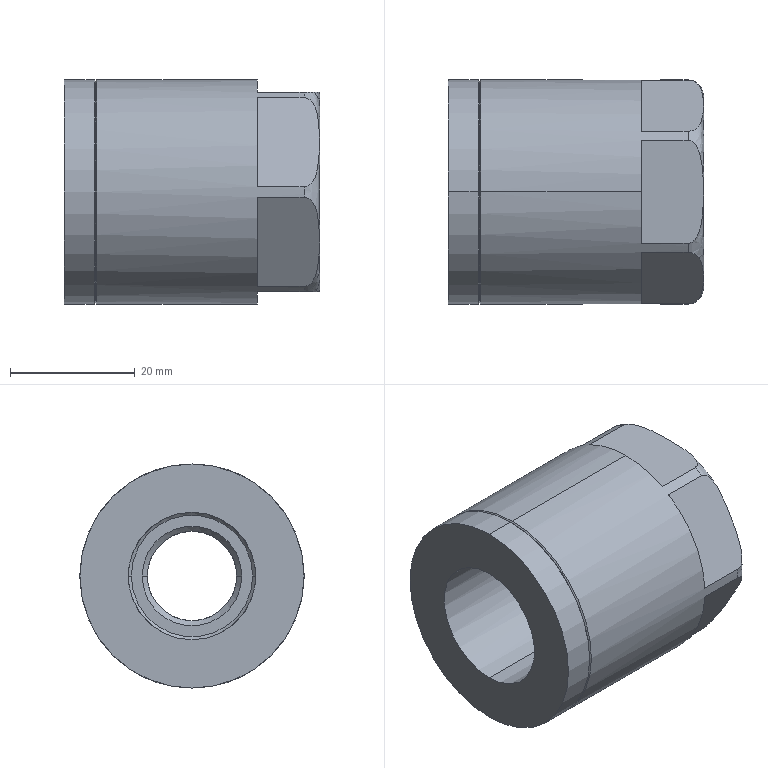Part | SolidWorks | features BaseBody 1 | 1 solid | 35 faces | box 41 x 36 x 36 mm | volume 28650 mm3 | plane 15 | cone 10 | cylinder 8 | spline 2 | commonest cylinder face diameters 36 x4 14.376 x2 20.5 x2
STEP:
#1=CARTESIAN_POINT('',(41.,0.,-15.5));
#2=VERTEX_POINT('',#1);
#3=CARTESIAN_POINT('',(41.,0.,15.5));
#4=VERTEX_POINT('',#3);
#5=CARTESIAN_POINT('',(41.,0.,-15.5));
#6=CARTESIAN_POINT('',(41.,-31.,-15.5));
#7=CARTESIAN_POINT('',(41.,-31.,15.5));
#8=CARTESIAN_POINT('',(41.,0.,15.5));
#9=(BOUNDED_CURVE()B_SPLINE_CURVE(3,(#5,#6,#7,#8),.UNSPECIFIED.,.F.,.F.)B_SPLINE_CURVE_WITH_KNOTS((4,4),(0.,0.5),.UNSPECIFIED.)CURVE()GEOMETRIC_REPRESENTATION_ITEM()RATIONAL_B_SPLINE_CURVE((1.,0.3333,0.3333,1.))REPRESENTATION_ITEM(''));
#10=EDGE_CURVE('',#2,#4,#9,.T.);
#11=ORIENTED_EDGE('',*,*,#10,.T.);
#12=CARTESIAN_POINT('',(40.949,0.,16.));
#13=VERTEX_POINT('',#12);
#14=CARTESIAN_POINT('',(38.5,0.,15.5));
#15=DIRECTION('',(0.,-1.,0.));
#16=DIRECTION('',(0.,0.,1.));
#17=AXIS2_PLACEMENT_3D('',#14,#15,#16);
#18=CIRCLE('',#17,2.5);
#19=EDGE_CURVE('',#4,#13,#18,.T.);
#20=ORIENTED_EDGE('',*,*,#19,.T.);
#21=CARTESIAN_POINT('',(38.5,-8.246,16.));
#22=VERTEX_POINT('',#21);
#23=CARTESIAN_POINT('',(38.5,-8.246,16.));
#24=CARTESIAN_POINT('',(38.598,-8.246,16.));
#25=CARTESIAN_POINT('',(38.694,-8.234,16.));
#26=CARTESIAN_POINT('',(38.882,-8.186,16.));
#27=CARTESIAN_POINT('',(38.974,-8.151,16.));
#28=CARTESIAN_POINT('',(39.233,-8.019,16.));
#29=CARTESIAN_POINT('',(39.388,-7.896,16.));
#30=CARTESIAN_POINT('',(39.657,-7.62,16.));
#31=CARTESIAN_POINT('',(39.774,-7.463,16.));
#32=CARTESIAN_POINT('',(39.98,-7.137,16.));
#33=CARTESIAN_POINT('',(40.068,-6.966,16.));
#34=CARTESIAN_POINT('',(40.303,-6.439,16.));
#35=CARTESIAN_POINT('',(40.42,-6.068,16.));
#36=CARTESIAN_POINT('',(40.604,-5.326,16.));
#37=CARTESIAN_POINT('',(40.671,-4.951,16.));
#38=CARTESIAN_POINT('',(40.831,-3.82,16.));
#39=CARTESIAN_POINT('',(40.881,-3.056,16.));
#40=CARTESIAN_POINT('',(40.94,-1.527,16.));
#41=CARTESIAN_POINT('',(40.949,-0.763,16.));
#42=CARTESIAN_POINT('',(40.949,0.,16.));
#43=B_SPLINE_CURVE_WITH_KNOTS('',3,(#23,#24,#25,#26,#27,#28,#29,#30,#31,#32,#33,#34,#35,#36,#37,#38,#39,#40,#41,#42),.UNSPECIFIED.,.F.,.F.,(4,2,2,2,2,2,2,2,2,4),(0.,0.0002896,0.0005792,0.001158,0.001738,0.002317,0.003475,0.004634,0.006951,0.009268),.UNSPECIFIED.);
#44=EDGE_CURVE('',#22,#13,#43,.T.);
#45=ORIENTED_EDGE('',*,*,#44,.F.);
#46=CARTESIAN_POINT('',(38.5,-9.733,15.141));
#47=VERTEX_POINT('',#46);
#48=CARTESIAN_POINT('',(38.5,0.,0.));
#49=DIRECTION('',(1.,0.,0.));
#50=DIRECTION('',(0.,0.,-1.));
#51=AXIS2_PLACEMENT_3D('',#48,#49,#50);
#52=CIRCLE('',#51,18.);
#53=EDGE_CURVE('',#22,#47,#52,.T.);
#54=ORIENTED_EDGE('',*,*,#53,.T.);
#55=CARTESIAN_POINT('',(38.5,-17.98,0.8586));
#56=VERTEX_POINT('',#55);
#57=CARTESIAN_POINT('',(38.5,-17.98,0.8586));
#58=CARTESIAN_POINT('',(38.598,-17.98,0.8586));
#59=CARTESIAN_POINT('',(38.694,-17.973,0.8694));
#60=CARTESIAN_POINT('',(38.881,-17.95,0.9105));
#61=CARTESIAN_POINT('',(38.973,-17.932,0.9412));
#62=CARTESIAN_POINT('',(39.232,-17.866,1.055));
#63=CARTESIAN_POINT('',(39.386,-17.805,1.161));
#64=CARTESIAN_POINT('',(39.655,-17.667,1.4));
#65=CARTESIAN_POINT('',(39.773,-17.589,1.535));
#66=CARTESIAN_POINT('',(39.978,-17.426,1.817));
#67=CARTESIAN_POINT('',(40.066,-17.341,1.964));
#68=CARTESIAN_POINT('',(40.302,-17.078,2.42));
#69=CARTESIAN_POINT('',(40.419,-16.893,2.74));
#70=CARTESIAN_POINT('',(40.602,-16.523,3.382));
#71=CARTESIAN_POINT('',(40.67,-16.336,3.706));
#72=CARTESIAN_POINT('',(40.83,-15.771,4.684));
#73=CARTESIAN_POINT('',(40.88,-15.389,5.345));
#74=CARTESIAN_POINT('',(40.94,-14.626,6.667));
#75=CARTESIAN_POINT('',(40.949,-14.245,7.327));
#76=CARTESIAN_POINT('',(40.95,-13.483,8.646));
#77=CARTESIAN_POINT('',(40.941,-13.103,9.305));
#78=CARTESIAN_POINT('',(40.882,-12.343,10.622));
#79=CARTESIAN_POINT('',(40.834,-11.963,11.28));
#80=CARTESIAN_POINT('',(40.676,-11.395,12.263));
#81=CARTESIAN_POINT('',(40.609,-11.207,12.59));
#82=CARTESIAN_POINT('',(40.425,-10.83,13.241));
#83=CARTESIAN_POINT('',(40.309,-10.644,13.564));
#84=CARTESIAN_POINT('',(40.072,-10.377,14.026));
#85=CARTESIAN_POINT('',(39.983,-10.291,14.175));
#86=CARTESIAN_POINT('',(39.779,-10.128,14.457));
#87=CARTESIAN_POINT('',(39.664,-10.051,14.591));
#88=CARTESIAN_POINT('',(39.392,-9.91,14.835));
#89=CARTESIAN_POINT('',(39.237,-9.848,14.942));
#90=CARTESIAN_POINT('',(38.976,-9.782,15.058));
#91=CARTESIAN_POINT('',(38.886,-9.764,15.088));
#92=CARTESIAN_POINT('',(38.698,-9.74,15.13));
#93=CARTESIAN_POINT('',(38.599,-9.733,15.141));
#94=CARTESIAN_POINT('',(38.5,-9.733,15.141));
#95=B_SPLINE_CURVE_WITH_KNOTS('',3,(#57,#58,#59,#60,#61,#62,#63,#64,#65,#66,#67,#68,#69,#70,#71,#72,#73,#74,#75,#76,#77,#78,#79,#80,#81,#82,#83,#84,#85,#86,#87,#88,#89,#90,#91,#92,#93,#94),.UNSPECIFIED.,.F.,.F.,(4,2,2,2,2,2,2,2,2,2,2,2,2,2,2,2,2,2,4),(0.,0.0002891,0.0005782,0.001156,0.001735,0.002313,0.003469,0.004626,0.006939,0.009252,0.01156,0.01388,0.01503,0.01619,0.01677,0.01735,0.01792,0.01821,0.0185),.UNSPECIFIED.);
#96=EDGE_CURVE('',#56,#47,#95,.T.);
#97=ORIENTED_EDGE('',*,*,#96,.F.);
#98=CARTESIAN_POINT('',(38.5,-17.98,-0.8586));
#99=VERTEX_POINT('',#98);
#100=CARTESIAN_POINT('',(38.5,0.,0.));
#101=DIRECTION('',(1.,0.,0.));
#102=DIRECTION('',(0.,0.,-1.));
#103=AXIS2_PLACEMENT_3D('',#100,#101,#102);
#104=CIRCLE('',#103,18.);
#105=EDGE_CURVE('',#56,#99,#104,.T.);
#106=ORIENTED_EDGE('',*,*,#105,.T.);
#107=CARTESIAN_POINT('',(38.5,-9.733,-15.141));
#108=VERTEX_POINT('',#107);
#109=CARTESIAN_POINT('',(38.5,-9.733,-15.141));
#110=CARTESIAN_POINT('',(38.598,-9.733,-15.141));
#111=CARTESIAN_POINT('',(38.694,-9.74,-15.131));
#112=CARTESIAN_POINT('',(38.881,-9.763,-15.09));
#113=CARTESIAN_POINT('',(38.973,-9.781,-15.059));
#114=CARTESIAN_POINT('',(39.232,-9.847,-14.945));
#115=CARTESIAN_POINT('',(39.386,-9.908,-14.839));
#116=CARTESIAN_POINT('',(39.655,-10.046,-14.6));
#117=CARTESIAN_POINT('',(39.773,-10.124,-14.465));
#118=CARTESIAN_POINT('',(39.978,-10.287,-14.183));
#119=CARTESIAN_POINT('',(40.066,-10.372,-14.036));
#120=CARTESIAN_POINT('',(40.302,-10.635,-13.58));
#121=CARTESIAN_POINT('',(40.419,-10.82,-13.26));
#122=CARTESIAN_POINT('',(40.602,-11.19,-12.618));
#123=CARTESIAN_POINT('',(40.67,-11.377,-12.294));
#124=CARTESIAN_POINT('',(40.83,-11.942,-11.316));
#125=CARTESIAN_POINT('',(40.88,-12.323,-10.655));
#126=CARTESIAN_POINT('',(40.94,-13.087,-9.333));
#127=CARTESIAN_POINT('',(40.949,-13.468,-8.673));
#128=CARTESIAN_POINT('',(40.95,-14.229,-7.354));
#129=CARTESIAN_POINT('',(40.941,-14.61,-6.695));
#130=CARTESIAN_POINT('',(40.882,-15.37,-5.378));
#131=CARTESIAN_POINT('',(40.834,-15.75,-4.72));
#132=CARTESIAN_POINT('',(40.676,-16.317,-3.737));
#133=CARTESIAN_POINT('',(40.609,-16.506,-3.41));
#134=CARTESIAN_POINT('',(40.425,-16.883,-2.759));
#135=CARTESIAN_POINT('',(40.309,-17.069,-2.436));
#136=CARTESIAN_POINT('',(40.072,-17.336,-1.974));
#137=CARTESIAN_POINT('',(39.983,-17.421,-1.825));
#138=CARTESIAN_POINT('',(39.779,-17.584,-1.543));
#139=CARTESIAN_POINT('',(39.664,-17.662,-1.409));
#140=CARTESIAN_POINT('',(39.392,-17.803,-1.165));
#141=CARTESIAN_POINT('',(39.237,-17.864,-1.058));
#142=CARTESIAN_POINT('',(38.976,-17.931,-0.9423));
#143=CARTESIAN_POINT('',(38.886,-17.949,-0.9119));
#144=CARTESIAN_POINT('',(38.698,-17.973,-0.8699));
#145=CARTESIAN_POINT('',(38.599,-17.98,-0.8586));
#146=CARTESIAN_POINT('',(38.5,-17.98,-0.8586));
#147=B_SPLINE_CURVE_WITH_KNOTS('',3,(#109,#110,#111,#112,#113,#114,#115,#116,#117,#118,#119,#120,#121,#122,#123,#124,#125,#126,#127,#128,#129,#130,#131,#132,#133,#134,#135,#136,#137,#138,#139,#140,#141,#142,#143,#144,#145,#146),.UNSPECIFIED.,.F.,.F.,(4,2,2,2,2,2,2,2,2,2,2,2,2,2,2,2,2,2,4),(0.,0.0002891,0.0005782,0.001156,0.001735,0.002313,0.003469,0.004626,0.006939,0.009252,0.01156,0.01388,0.01503,0.01619,0.01677,0.01735,0.01792,0.01821,0.0185),.UNSPECIFIED.);
#148=EDGE_CURVE('',#108,#99,#147,.T.);
#149=ORIENTED_EDGE('',*,*,#148,.F.);
#150=CARTESIAN_POINT('',(38.5,-8.246,-16.));
#151=VERTEX_POINT('',#150);
#152=CARTESIAN_POINT('',(38.5,0.,0.));
#153=DIRECTION('',(1.,0.,0.));
#154=DIRECTION('',(0.,0.,-1.));
#155=AXIS2_PLACEMENT_3D('',#152,#153,#154);
#156=CIRCLE('',#155,18.);
#157=EDGE_CURVE('',#108,#151,#156,.T.);
#158=ORIENTED_EDGE('',*,*,#157,.T.);
#159=CARTESIAN_POINT('',(40.949,0.,-16.));
#160=VERTEX_POINT('',#159);
#161=CARTESIAN_POINT('',(40.949,0.,-16.));
#162=CARTESIAN_POINT('',(40.949,-0.7604,-16.));
#163=CARTESIAN_POINT('',(40.94,-1.52,-16.));
#164=CARTESIAN_POINT('',(40.882,-3.038,-16.));
#165=CARTESIAN_POINT('',(40.833,-3.796,-16.));
#166=CARTESIAN_POINT('',(40.675,-4.929,-16.));
#167=CARTESIAN_POINT('',(40.608,-5.306,-16.));
#168=CARTESIAN_POINT('',(40.423,-6.058,-16.));
#169=CARTESIAN_POINT('',(40.307,-6.429,-16.));
#170=CARTESIAN_POINT('',(40.07,-6.962,-16.));
#171=CARTESIAN_POINT('',(39.982,-7.133,-16.));
#172=CARTESIAN_POINT('',(39.778,-7.458,-16.));
#173=CARTESIAN_POINT('',(39.663,-7.612,-16.));
#174=CARTESIAN_POINT('',(39.391,-7.893,-16.));
#175=CARTESIAN_POINT('',(39.236,-8.017,-16.));
#176=CARTESIAN_POINT('',(38.975,-8.15,-16.));
#177=CARTESIAN_POINT('',(38.885,-8.185,-16.));
#178=CARTESIAN_POINT('',(38.697,-8.233,-16.));
#179=CARTESIAN_POINT('',(38.599,-8.246,-16.));
#180=CARTESIAN_POINT('',(38.5,-8.246,-16.));
#181=B_SPLINE_CURVE_WITH_KNOTS('',3,(#161,#162,#163,#164,#165,#166,#167,#168,#169,#170,#171,#172,#173,#174,#175,#176,#177,#178,#179,#180),.UNSPECIFIED.,.F.,.F.,(4,2,2,2,2,2,2,2,2,4),(0.009268,0.01158,0.01389,0.01504,0.01619,0.01677,0.01735,0.01793,0.01821,0.0185),.UNSPECIFIED.);
#182=EDGE_CURVE('',#160,#151,#181,.T.);
#183=ORIENTED_EDGE('',*,*,#182,.F.);
#184=CARTESIAN_POINT('',(38.5,0.,-15.5));
#185=DIRECTION('',(0.,1.,0.));
#186=DIRECTION('',(0.,0.,-1.));
#187=AXIS2_PLACEMENT_3D('',#184,#185,#186);
#188=CIRCLE('',#187,2.5);
#189=EDGE_CURVE('',#2,#160,#188,.T.);
#190=ORIENTED_EDGE('',*,*,#189,.F.);
#191=EDGE_LOOP('',(#11,#20,#45,#54,#97,#106,#149,#158,#183,#190));
#192=FACE_OUTER_BOUND('',#191,.T.);
#193=CARTESIAN_POINT('',(40.994,0.,15.334));
#194=CARTESIAN_POINT('',(40.994,-30.667,15.334));
#195=CARTESIAN_POINT('',(40.994,-30.667,-15.334));
#196=CARTESIAN_POINT('',(40.994,0.,-15.334));
#197=CARTESIAN_POINT('',(41.097,0.,16.873));
#198=CARTESIAN_POINT('',(41.097,-33.746,16.873));
#199=CARTESIAN_POINT('',(41.097,-33.746,-16.873));
#200=CARTESIAN_POINT('',(41.097,0.,-16.873));
#201=CARTESIAN_POINT('',(40.043,0.,18.));
#202=CARTESIAN_POINT('',(40.043,-36.,18.));
#203=CARTESIAN_POINT('',(40.043,-36.,-18.));
#204=CARTESIAN_POINT('',(40.043,0.,-18.));
#205=CARTESIAN_POINT('',(38.5,0.,18.));
#206=CARTESIAN_POINT('',(38.5,-36.,18.));
#207=CARTESIAN_POINT('',(38.5,-36.,-18.));
#208=CARTESIAN_POINT('',(38.5,0.,-18.));
#209=(BOUNDED_SURFACE()B_SPLINE_SURFACE(3,3,((#193,#194,#195,#196),(#197,#198,#199,#200),(#201,#202,#203,#204),(#205,#206,#207,#208)),.UNSPECIFIED.,.F.,.F.,.T.)B_SPLINE_SURFACE_WITH_KNOTS((4,4),(4,4),(0.,1.),(0.,1.),.UNSPECIFIED.)GEOMETRIC_REPRESENTATION_ITEM()RATIONAL_B_SPLINE_SURFACE(((1.,0.3333,0.3333,1.),(0.7888,0.2629,0.2629,0.7888),(0.7888,0.2629,0.2629,0.7888),(1.,0.3333,0.3333,1.)))REPRESENTATION_ITEM('')SURFACE());
#210=ADVANCED_FACE('',(#192),#209,.T.);
#211=CARTESIAN_POINT('',(31.,8.246,-16.));
#212=VERTEX_POINT('',#211);
#213=CARTESIAN_POINT('',(31.,0.,-18.));
#214=VERTEX_POINT('',#213);
#215=CARTESIAN_POINT('',(31.,0.,0.));
#216=DIRECTION('',(-1.,0.,0.));
#217=DIRECTION('',(0.,0.,1.));
#218=AXIS2_PLACEMENT_3D('',#215,#216,#217);
#219=CIRCLE('',#218,18.);
#220=EDGE_CURVE('',#212,#214,#219,.T.);
#221=ORIENTED_EDGE('',*,*,#220,.T.);
#222=CARTESIAN_POINT('',(5.2,0.,-18.));
#223=VERTEX_POINT('',#222);
#224=CARTESIAN_POINT('',(41.,0.,-18.));
#225=DIRECTION('',(-1.,0.,0.));
#226=VECTOR('',#225,1000.);
#227=LINE('',#224,#226);
#228=EDGE_CURVE('',#214,#223,#227,.T.);
#229=ORIENTED_EDGE('',*,*,#228,.T.);
#230=CARTESIAN_POINT('',(5.2,0.,18.));
#231=VERTEX_POINT('',#230);
#232=CARTESIAN_POINT('',(5.2,0.,0.));
#233=DIRECTION('',(1.,0.,0.));
#234=DIRECTION('',(0.,0.,1.));
#235=AXIS2_PLACEMENT_3D('',#232,#233,#234);
#236=CIRCLE('',#235,18.);
#237=EDGE_CURVE('',#223,#231,#236,.T.);
#238=ORIENTED_EDGE('',*,*,#237,.T.);
#239=CARTESIAN_POINT('',(31.,0.,18.));
#240=VERTEX_POINT('',#239);
#241=CARTESIAN_POINT('',(41.,0.,18.));
#242=DIRECTION('',(-1.,0.,0.));
#243=VECTOR('',#242,1000.);
#244=LINE('',#241,#243);
#245=EDGE_CURVE('',#240,#231,#244,.T.);
#246=ORIENTED_EDGE('',*,*,#245,.F.);
#247=CARTESIAN_POINT('',(31.,8.246,16.));
#248=VERTEX_POINT('',#247);
#249=CARTESIAN_POINT('',(31.,0.,0.));
#250=DIRECTION('',(-1.,0.,0.));
#251=DIRECTION('',(0.,0.,1.));
#252=AXIS2_PLACEMENT_3D('',#249,#250,#251);
#253=CIRCLE('',#252,18.);
#254=EDGE_CURVE('',#240,#248,#253,.T.);
#255=ORIENTED_EDGE('',*,*,#254,.T.);
#256=CARTESIAN_POINT('',(38.5,8.246,16.));
#257=VERTEX_POINT('',#256);
#258=CARTESIAN_POINT('',(41.,8.246,16.));
#259=DIRECTION('',(1.,0.,0.));
#260=VECTOR('',#259,1000.);
#261=LINE('',#258,#260);
#262=EDGE_CURVE('',#248,#257,#261,.T.);
#263=ORIENTED_EDGE('',*,*,#262,.T.);
#264=CARTESIAN_POINT('',(38.5,9.733,15.141));
#265=VERTEX_POINT('',#264);
#266=CARTESIAN_POINT('',(38.5,0.,0.));
#267=DIRECTION('',(1.,0.,0.));
#268=DIRECTION('',(0.,0.,-1.));
#269=AXIS2_PLACEMENT_3D('',#266,#267,#268);
#270=CIRCLE('',#269,18.);
#271=EDGE_CURVE('',#265,#257,#270,.T.);
#272=ORIENTED_EDGE('',*,*,#271,.F.);
#273=CARTESIAN_POINT('',(31.,9.733,15.141));
#274=VERTEX_POINT('',#273);
#275=CARTESIAN_POINT('',(41.,9.733,15.141));
#276=DIRECTION('',(-1.,0.,0.));
#277=VECTOR('',#276,1000.);
#278=LINE('',#275,#277);
#279=EDGE_CURVE('',#265,#274,#278,.T.);
#280=ORIENTED_EDGE('',*,*,#279,.T.);
#281=CARTESIAN_POINT('',(31.,17.98,0.8586));
#282=VERTEX_POINT('',#281);
#283=CARTESIAN_POINT('',(31.,0.,0.));
#284=DIRECTION('',(-1.,0.,0.));
#285=DIRECTION('',(0.,0.,1.));
#286=AXIS2_PLACEMENT_3D('',#283,#284,#285);
#287=CIRCLE('',#286,18.);
#288=EDGE_CURVE('',#274,#282,#287,.T.);
#289=ORIENTED_EDGE('',*,*,#288,.T.);
#290=CARTESIAN_POINT('',(38.5,17.98,0.8586));
#291=VERTEX_POINT('',#290);
#292=CARTESIAN_POINT('',(41.,17.98,0.8586));
#293=DIRECTION('',(1.,0.,0.));
#294=VECTOR('',#293,1000.);
#295=LINE('',#292,#294);
#296=EDGE_CURVE('',#282,#291,#295,.T.);
#297=ORIENTED_EDGE('',*,*,#296,.T.);
#298=CARTESIAN_POINT('',(38.5,17.98,-0.8586));
#299=VERTEX_POINT('',#298);
#300=CARTESIAN_POINT('',(38.5,0.,0.));
#301=DIRECTION('',(1.,0.,0.));
#302=DIRECTION('',(0.,0.,-1.));
#303=AXIS2_PLACEMENT_3D('',#300,#301,#302);
#304=CIRCLE('',#303,18.);
#305=EDGE_CURVE('',#299,#291,#304,.T.);
#306=ORIENTED_EDGE('',*,*,#305,.F.);
#307=CARTESIAN_POINT('',(31.,17.98,-0.8586));
#308=VERTEX_POINT('',#307);
#309=CARTESIAN_POINT('',(41.,17.98,-0.8586));
#310=DIRECTION('',(-1.,0.,0.));
#311=VECTOR('',#310,1000.);
#312=LINE('',#309,#311);
#313=EDGE_CURVE('',#299,#308,#312,.T.);
#314=ORIENTED_EDGE('',*,*,#313,.T.);
#315=CARTESIAN_POINT('',(31.,9.733,-15.141));
#316=VERTEX_POINT('',#315);
#317=CARTESIAN_POINT('',(31.,0.,0.));
#318=DIRECTION('',(-1.,0.,0.));
#319=DIRECTION('',(0.,0.,1.));
#320=AXIS2_PLACEMENT_3D('',#317,#318,#319);
#321=CIRCLE('',#320,18.);
#322=EDGE_CURVE('',#308,#316,#321,.T.);
#323=ORIENTED_EDGE('',*,*,#322,.T.);
#324=CARTESIAN_POINT('',(38.5,9.733,-15.141));
#325=VERTEX_POINT('',#324);
#326=CARTESIAN_POINT('',(41.,9.733,-15.141));
#327=DIRECTION('',(1.,0.,0.));
#328=VECTOR('',#327,1000.);
#329=LINE('',#326,#328);
#330=EDGE_CURVE('',#316,#325,#329,.T.);
#331=ORIENTED_EDGE('',*,*,#330,.T.);
#332=CARTESIAN_POINT('',(38.5,8.246,-16.));
#333=VERTEX_POINT('',#332);
#334=CARTESIAN_POINT('',(38.5,0.,0.));
#335=DIRECTION('',(1.,0.,0.));
#336=DIRECTION('',(0.,0.,-1.));
#337=AXIS2_PLACEMENT_3D('',#334,#335,#336);
#338=CIRCLE('',#337,18.);
#339=EDGE_CURVE('',#333,#325,#338,.T.);
#340=ORIENTED_EDGE('',*,*,#339,.F.);
#341=CARTESIAN_POINT('',(41.,8.246,-16.));
#342=DIRECTION('',(-1.,0.,0.));
#343=VECTOR('',#342,1000.);
#344=LINE('',#341,#343);
#345=EDGE_CURVE('',#333,#212,#344,.T.);
#346=ORIENTED_EDGE('',*,*,#345,.T.);
#347=EDGE_LOOP('',(#221,#229,#238,#246,#255,#263,#272,#280,#289,#297,#306,#314,#323,#331,#340,#346));
#348=FACE_OUTER_BOUND('',#347,.T.);
#349=CARTESIAN_POINT('',(41.,0.,0.));
#350=DIRECTION('',(-1.,0.,0.));
#351=DIRECTION('',(0.,0.,1.));
#352=AXIS2_PLACEMENT_3D('',#349,#350,#351);
#353=CYLINDRICAL_SURFACE('',#352,18.);
#354=ADVANCED_FACE('',(#348),#353,.T.);
#355=CARTESIAN_POINT('',(5.,0.,-17.8));
#356=VERTEX_POINT('',#355);
#357=CARTESIAN_POINT('',(5.,0.,17.8));
#358=VERTEX_POINT('',#357);
#359=CARTESIAN_POINT('',(5.,0.,0.));
#360=DIRECTION('',(1.,0.,0.));
#361=DIRECTION('',(0.,0.,-1.));
#362=AXIS2_PLACEMENT_3D('',#359,#360,#361);
#363=CIRCLE('',#362,17.8);
#364=EDGE_CURVE('',#356,#358,#363,.T.);
#365=ORIENTED_EDGE('',*,*,#364,.T.);
#366=CARTESIAN_POINT('',(5.2,0.,18.));
#367=DIRECTION('',(0.7071,0.,0.7071));
#368=VECTOR('',#367,1000.);
#369=LINE('',#366,#368);
#370=EDGE_CURVE('',#358,#231,#369,.T.);
#371=ORIENTED_EDGE('',*,*,#370,.T.);
#372=ORIENTED_EDGE('',*,*,#237,.F.);
#373=CARTESIAN_POINT('',(5.2,0.,-18.));
#374=DIRECTION('',(0.7071,0.,-0.7071));
#375=VECTOR('',#374,1000.);
#376=LINE('',#373,#375);
#377=EDGE_CURVE('',#356,#223,#376,.T.);
#378=ORIENTED_EDGE('',*,*,#377,.F.);
#379=EDGE_LOOP('',(#365,#371,#372,#378));
#380=FACE_OUTER_BOUND('',#379,.T.);
#381=CARTESIAN_POINT('',(5.2,0.,0.));
#382=DIRECTION('',(1.,0.,0.));
#383=DIRECTION('',(0.,0.,-1.));
#384=AXIS2_PLACEMENT_3D('',#381,#382,#383);
#385=CONICAL_SURFACE('',#384,18.,0.7854);
#386=ADVANCED_FACE('',(#380),#385,.T.);
#387=ORIENTED_EDGE('',*,*,#364,.F.);
#388=CARTESIAN_POINT('',(4.8,0.,-18.));
#389=VERTEX_POINT('',#388);
#390=CARTESIAN_POINT('',(4.8,0.,-18.));
#391=DIRECTION('',(-0.7071,0.,-0.7071));
#392=VECTOR('',#391,1000.);
#393=LINE('',#390,#392);
#394=EDGE_CURVE('',#356,#389,#393,.T.);
#395=ORIENTED_EDGE('',*,*,#394,.T.);
#396=CARTESIAN_POINT('',(4.8,0.,18.));
#397=VERTEX_POINT('',#396);
#398=CARTESIAN_POINT('',(4.8,0.,0.));
#399=DIRECTION('',(1.,0.,0.));
#400=DIRECTION('',(0.,0.,1.));
#401=AXIS2_PLACEMENT_3D('',#398,#399,#400);
#402=CIRCLE('',#401,18.);
#403=EDGE_CURVE('',#389,#397,#402,.T.);
#404=ORIENTED_EDGE('',*,*,#403,.T.);
#405=CARTESIAN_POINT('',(4.8,0.,18.));
#406=DIRECTION('',(-0.7071,0.,0.7071));
#407=VECTOR('',#406,1000.);
#408=LINE('',#405,#407);
#409=EDGE_CURVE('',#358,#397,#408,.T.);
#410=ORIENTED_EDGE('',*,*,#409,.F.);
#411=EDGE_LOOP('',(#387,#395,#404,#410));
#412=FACE_OUTER_BOUND('',#411,.T.);
#413=CARTESIAN_POINT('',(4.8,0.,0.));
#414=DIRECTION('',(-1.,0.,0.));
#415=DIRECTION('',(0.,0.,1.));
#416=AXIS2_PLACEMENT_3D('',#413,#414,#415);
#417=CONICAL_SURFACE('',#416,18.,0.7854);
#418=ADVANCED_FACE('',(#412),#417,.T.);
#419=ORIENTED_EDGE('',*,*,#403,.F.);
#420=CARTESIAN_POINT('',(0.,0.,-18.));
#421=VERTEX_POINT('',#420);
#422=CARTESIAN_POINT('',(41.,0.,-18.));
#423=DIRECTION('',(-1.,0.,0.));
#424=VECTOR('',#423,1000.);
#425=LINE('',#422,#424);
#426=EDGE_CURVE('',#389,#421,#425,.T.);
#427=ORIENTED_EDGE('',*,*,#426,.T.);
#428=CARTESIAN_POINT('',(0.,0.,18.));
#429=VERTEX_POINT('',#428);
#430=CARTESIAN_POINT('',(0.,0.,0.));
#431=DIRECTION('',(1.,0.,0.));
#432=DIRECTION('',(0.,0.,1.));
#433=AXIS2_PLACEMENT_3D('',#430,#431,#432);
#434=CIRCLE('',#433,18.);
#435=EDGE_CURVE('',#421,#429,#434,.T.);
#436=ORIENTED_EDGE('',*,*,#435,.T.);
#437=CARTESIAN_POINT('',(41.,0.,18.));
#438=DIRECTION('',(-1.,0.,0.));
#439=VECTOR('',#438,1000.);
#440=LINE('',#437,#439);
#441=EDGE_CURVE('',#397,#429,#440,.T.);
#442=ORIENTED_EDGE('',*,*,#441,.F.);
#443=EDGE_LOOP('',(#419,#427,#436,#442));
#444=FACE_OUTER_BOUND('',#443,.T.);
#445=CARTESIAN_POINT('',(41.,0.,0.));
#446=DIRECTION('',(-1.,0.,0.));
#447=DIRECTION('',(0.,0.,1.));
#448=AXIS2_PLACEMENT_3D('',#445,#446,#447);
#449=CYLINDRICAL_SURFACE('',#448,18.);
#450=ADVANCED_FACE('',(#444),#449,.T.);
#451=CARTESIAN_POINT('',(40.188,0.,7.188));
#452=VERTEX_POINT('',#451);
#453=CARTESIAN_POINT('',(40.188,0.,-7.188));
#454=VERTEX_POINT('',#453);
#455=CARTESIAN_POINT('',(40.188,0.,0.));
#456=DIRECTION('',(1.,0.,0.));
#457=DIRECTION('',(0.,0.,-1.));
#458=AXIS2_PLACEMENT_3D('',#455,#456,#457);
#459=CIRCLE('',#458,7.188);
#460=EDGE_CURVE('',#452,#454,#459,.T.);
#461=ORIENTED_EDGE('',*,*,#460,.F.);
#462=CARTESIAN_POINT('',(41.,0.,8.));
#463=VERTEX_POINT('',#462);
#464=CARTESIAN_POINT('',(41.,0.,8.));
#465=DIRECTION('',(0.7071,0.,0.7071));
#466=VECTOR('',#465,1000.);
#467=LINE('',#464,#466);
#468=EDGE_CURVE('',#452,#463,#467,.T.);
#469=ORIENTED_EDGE('',*,*,#468,.T.);
#470=CARTESIAN_POINT('',(41.,0.,-8.));
#471=VERTEX_POINT('',#470);
#472=CARTESIAN_POINT('',(41.,0.,0.));
#473=DIRECTION('',(1.,0.,0.));
#474=DIRECTION('',(0.,0.,-1.));
#475=AXIS2_PLACEMENT_3D('',#472,#473,#474);
#476=CIRCLE('',#475,8.);
#477=EDGE_CURVE('',#463,#471,#476,.T.);
#478=ORIENTED_EDGE('',*,*,#477,.T.);
#479=CARTESIAN_POINT('',(41.,0.,-8.));
#480=DIRECTION('',(0.7071,0.,-0.7071));
#481=VECTOR('',#480,1000.);
#482=LINE('',#479,#481);
#483=EDGE_CURVE('',#454,#471,#482,.T.);
#484=ORIENTED_EDGE('',*,*,#483,.F.);
#485=EDGE_LOOP('',(#461,#469,#478,#484));
#486=FACE_OUTER_BOUND('',#485,.T.);
#487=CARTESIAN_POINT('',(41.,0.,0.));
#488=DIRECTION('',(1.,0.,0.));
#489=DIRECTION('',(0.,0.,-1.));
#490=AXIS2_PLACEMENT_3D('',#487,#488,#489);
#491=CONICAL_SURFACE('',#490,8.,0.7854);
#492=ADVANCED_FACE('',(#486),#491,.F.);
#493=CARTESIAN_POINT('',(29.5,0.,-10.25));
#494=VERTEX_POINT('',#493);
#495=CARTESIAN_POINT('',(29.5,-10.25,0.));
#496=VERTEX_POINT('',#495);
#497=CARTESIAN_POINT('',(29.5,0.,0.));
#498=DIRECTION('',(-1.,0.,0.));
#499=DIRECTION('',(0.,0.,1.));
#500=AXIS2_PLACEMENT_3D('',#497,#498,#499);
#501=CIRCLE('',#500,10.25);
#502=EDGE_CURVE('',#494,#496,#501,.T.);
#503=ORIENTED_EDGE('',*,*,#502,.F.);
#504=CARTESIAN_POINT('',(0.,0.,-10.25));
#505=VERTEX_POINT('',#504);
#506=CARTESIAN_POINT('',(41.,0.,-10.25));
#507=DIRECTION('',(-1.,0.,0.));
#508=VECTOR('',#507,1000.);
#509=LINE('',#506,#508);
#510=EDGE_CURVE('',#494,#505,#509,.T.);
#511=ORIENTED_EDGE('',*,*,#510,.T.);
#512=CARTESIAN_POINT('',(0.,0.,10.25));
#513=VERTEX_POINT('',#512);
#514=CARTESIAN_POINT('',(0.,0.,0.));
#515=DIRECTION('',(-1.,0.,0.));
#516=DIRECTION('',(0.,0.,1.));
#517=AXIS2_PLACEMENT_3D('',#514,#515,#516);
#518=CIRCLE('',#517,10.25);
#519=EDGE_CURVE('',#505,#513,#518,.T.);
#520=ORIENTED_EDGE('',*,*,#519,.T.);
#521=CARTESIAN_POINT('',(29.5,0.,10.25));
#522=VERTEX_POINT('',#521);
#523=CARTESIAN_POINT('',(41.,0.,10.25));
#524=DIRECTION('',(-1.,0.,0.));
#525=VECTOR('',#524,1000.);
#526=LINE('',#523,#525);
#527=EDGE_CURVE('',#522,#513,#526,.T.);
#528=ORIENTED_EDGE('',*,*,#527,.F.);
#529=CARTESIAN_POINT('',(29.5,0.,0.));
#530=DIRECTION('',(-1.,0.,0.));
#531=DIRECTION('',(0.,0.,1.));
#532=AXIS2_PLACEMENT_3D('',#529,#530,#531);
#533=CIRCLE('',#532,10.25);
#534=EDGE_CURVE('',#496,#522,#533,.T.);
#535=ORIENTED_EDGE('',*,*,#534,.F.);
#536=EDGE_LOOP('',(#503,#511,#520,#528,#535));
#537=FACE_OUTER_BOUND('',#536,.T.);
#538=CARTESIAN_POINT('',(41.,0.,0.));
#539=DIRECTION('',(-1.,0.,0.));
#540=DIRECTION('',(0.,0.,1.));
#541=AXIS2_PLACEMENT_3D('',#538,#539,#540);
#542=CYLINDRICAL_SURFACE('',#541,10.25);
#543=ADVANCED_FACE('',(#537),#542,.F.);
#544=ORIENTED_EDGE('',*,*,#460,.T.);
#545=CARTESIAN_POINT('',(30.812,0.,-7.188));
#546=VERTEX_POINT('',#545);
#547=CARTESIAN_POINT('',(41.,0.,-7.188));
#548=DIRECTION('',(-1.,0.,0.));
#549=VECTOR('',#548,1000.);
#550=LINE('',#547,#549);
#551=EDGE_CURVE('',#454,#546,#550,.T.);
#552=ORIENTED_EDGE('',*,*,#551,.T.);
#553=CARTESIAN_POINT('',(30.812,-7.188,0.));
#554=VERTEX_POINT('',#553);
#555=CARTESIAN_POINT('',(30.812,0.,0.));
#556=DIRECTION('',(1.,0.,0.));
#557=DIRECTION('',(0.,0.,1.));
#558=AXIS2_PLACEMENT_3D('',#555,#556,#557);
#559=CIRCLE('',#558,7.188);
#560=EDGE_CURVE('',#554,#546,#559,.T.);
#561=ORIENTED_EDGE('',*,*,#560,.F.);
#562=CARTESIAN_POINT('',(30.812,0.,7.188));
#563=VERTEX_POINT('',#562);
#564=CARTESIAN_POINT('',(30.812,0.,0.));
#565=DIRECTION('',(1.,0.,0.));
#566=DIRECTION('',(0.,0.,1.));
#567=AXIS2_PLACEMENT_3D('',#564,#565,#566);
#568=CIRCLE('',#567,7.188);
#569=EDGE_CURVE('',#563,#554,#568,.T.);
#570=ORIENTED_EDGE('',*,*,#569,.F.);
#571=CARTESIAN_POINT('',(41.,0.,7.188));
#572=DIRECTION('',(-1.,0.,0.));
#573=VECTOR('',#572,1000.);
#574=LINE('',#571,#573);
#575=EDGE_CURVE('',#452,#563,#574,.T.);
#576=ORIENTED_EDGE('',*,*,#575,.F.);
#577=EDGE_LOOP('',(#544,#552,#561,#570,#576));
#578=FACE_OUTER_BOUND('',#577,.T.);
#579=CARTESIAN_POINT('',(41.,0.,0.));
#580=DIRECTION('',(-1.,0.,0.));
#581=DIRECTION('',(0.,0.,1.));
#582=AXIS2_PLACEMENT_3D('',#579,#580,#581);
#583=CYLINDRICAL_SURFACE('',#582,7.188);
#584=ADVANCED_FACE('',(#578),#583,.F.);
#585=CARTESIAN_POINT('',(30.,9.75,0.));
#586=VERTEX_POINT('',#585);
#587=CARTESIAN_POINT('',(30.,-9.75,0.));
#588=VERTEX_POINT('',#587);
#589=CARTESIAN_POINT('',(30.,0.,0.));
#590=DIRECTION('',(-1.,0.,0.));
#591=DIRECTION('',(0.,-1.,0.));
#592=AXIS2_PLACEMENT_3D('',#589,#590,#591);
#593=CIRCLE('',#592,9.75);
#594=EDGE_CURVE('',#586,#588,#593,.T.);
#595=ORIENTED_EDGE('',*,*,#594,.F.);
#596=CARTESIAN_POINT('',(29.5,10.25,0.));
#597=VERTEX_POINT('',#596);
#598=CARTESIAN_POINT('',(29.5,10.25,0.));
#599=DIRECTION('',(-0.7071,0.7071,0.));
#600=VECTOR('',#599,1000.);
#601=LINE('',#598,#600);
#602=EDGE_CURVE('',#586,#597,#601,.T.);
#603=ORIENTED_EDGE('',*,*,#602,.T.);
#604=CARTESIAN_POINT('',(29.5,0.,0.));
#605=DIRECTION('',(-1.,0.,0.));
#606=DIRECTION('',(0.,0.,1.));
#607=AXIS2_PLACEMENT_3D('',#604,#605,#606);
#608=CIRCLE('',#607,10.25);
#609=EDGE_CURVE('',#597,#494,#608,.T.);
#610=ORIENTED_EDGE('',*,*,#609,.T.);
#611=ORIENTED_EDGE('',*,*,#502,.T.);
#612=CARTESIAN_POINT('',(29.5,-10.25,0.));
#613=DIRECTION('',(-0.7071,-0.7071,0.));
#614=VECTOR('',#613,1000.);
#615=LINE('',#612,#614);
#616=EDGE_CURVE('',#588,#496,#615,.T.);
#617=ORIENTED_EDGE('',*,*,#616,.F.);
#618=EDGE_LOOP('',(#595,#603,#610,#611,#617));
#619=FACE_OUTER_BOUND('',#618,.T.);
#620=CARTESIAN_POINT('',(29.5,0.,0.));
#621=DIRECTION('',(-1.,0.,0.));
#622=DIRECTION('',(0.,-1.,0.));
#623=AXIS2_PLACEMENT_3D('',#620,#621,#622);
#624=CONICAL_SURFACE('',#623,10.25,0.7854);
#625=ADVANCED_FACE('',(#619),#624,.F.);
#626=ORIENTED_EDGE('',*,*,#560,.T.);
#627=CARTESIAN_POINT('',(30.812,7.188,0.));
#628=VERTEX_POINT('',#627);
#629=CARTESIAN_POINT('',(30.812,0.,0.));
#630=DIRECTION('',(1.,0.,0.));
#631=DIRECTION('',(0.,0.,1.));
#632=AXIS2_PLACEMENT_3D('',#629,#630,#631);
#633=CIRCLE('',#632,7.188);
#634=EDGE_CURVE('',#546,#628,#633,.T.);
#635=ORIENTED_EDGE('',*,*,#634,.T.);
#636=CARTESIAN_POINT('',(30.,8.,0.));
#637=VERTEX_POINT('',#636);
#638=CARTESIAN_POINT('',(30.,8.,0.));
#639=DIRECTION('',(-0.7071,0.7071,0.));
#640=VECTOR('',#639,1000.);
#641=LINE('',#638,#640);
#642=EDGE_CURVE('',#628,#637,#641,.T.);
#643=ORIENTED_EDGE('',*,*,#642,.T.);
#644=CARTESIAN_POINT('',(30.,-8.,0.));
#645=VERTEX_POINT('',#644);
#646=CARTESIAN_POINT('',(30.,0.,0.));
#647=DIRECTION('',(1.,0.,0.));
#648=DIRECTION('',(0.,-1.,0.));
#649=AXIS2_PLACEMENT_3D('',#646,#647,#648);
#650=CIRCLE('',#649,8.);
#651=EDGE_CURVE('',#645,#637,#650,.T.);
#652=ORIENTED_EDGE('',*,*,#651,.F.);
#653=CARTESIAN_POINT('',(30.,-8.,0.));
#654=DIRECTION('',(-0.7071,-0.7071,0.));
#655=VECTOR('',#654,1000.);
#656=LINE('',#653,#655);
#657=EDGE_CURVE('',#554,#645,#656,.T.);
#658=ORIENTED_EDGE('',*,*,#657,.F.);
#659=EDGE_LOOP('',(#626,#635,#643,#652,#658));
#660=FACE_OUTER_BOUND('',#659,.T.);
#661=CARTESIAN_POINT('',(30.,0.,0.));
#662=DIRECTION('',(-1.,0.,0.));
#663=DIRECTION('',(0.,-1.,0.));
#664=AXIS2_PLACEMENT_3D('',#661,#662,#663);
#665=CONICAL_SURFACE('',#664,8.,0.7854);
#666=ADVANCED_FACE('',(#660),#665,.F.);
#667=ORIENTED_EDGE('',*,*,#228,.F.);
#668=CARTESIAN_POINT('',(31.,-8.246,-16.));
#669=VERTEX_POINT('',#668);
#670=CARTESIAN_POINT('',(31.,0.,0.));
#671=DIRECTION('',(-1.,0.,0.));
#672=DIRECTION('',(0.,0.,1.));
#673=AXIS2_PLACEMENT_3D('',#670,#671,#672);
#674=CIRCLE('',#673,18.);
#675=EDGE_CURVE('',#214,#669,#674,.T.);
#676=ORIENTED_EDGE('',*,*,#675,.T.);
#677=CARTESIAN_POINT('',(41.,-8.246,-16.));
#678=DIRECTION('',(1.,0.,0.));
#679=VECTOR('',#678,1000.);
#680=LINE('',#677,#679);
#681=EDGE_CURVE('',#669,#151,#680,.T.);
#682=ORIENTED_EDGE('',*,*,#681,.T.);
#683=ORIENTED_EDGE('',*,*,#157,.F.);
#684=CARTESIAN_POINT('',(31.,-9.733,-15.141));
#685=VERTEX_POINT('',#684);
#686=CARTESIAN_POINT('',(41.,-9.733,-15.141));
#687=DIRECTION('',(-1.,0.,0.));
#688=VECTOR('',#687,1000.);
#689=LINE('',#686,#688);
#690=EDGE_CURVE('',#108,#685,#689,.T.);
#691=ORIENTED_EDGE('',*,*,#690,.T.);
#692=CARTESIAN_POINT('',(31.,-17.98,-0.8586));
#693=VERTEX_POINT('',#692);
#694=CARTESIAN_POINT('',(31.,0.,0.));
#695=DIRECTION('',(-1.,0.,0.));
#696=DIRECTION('',(0.,0.,1.));
#697=AXIS2_PLACEMENT_3D('',#694,#695,#696);
#698=CIRCLE('',#697,18.);
#699=EDGE_CURVE('',#685,#693,#698,.T.);
#700=ORIENTED_EDGE('',*,*,#699,.T.);
#701=CARTESIAN_POINT('',(41.,-17.98,-0.8586));
#702=DIRECTION('',(1.,0.,0.));
#703=VECTOR('',#702,1000.);
#704=LINE('',#701,#703);
#705=EDGE_CURVE('',#693,#99,#704,.T.);
#706=ORIENTED_EDGE('',*,*,#705,.T.);
#707=ORIENTED_EDGE('',*,*,#105,.F.);
#708=CARTESIAN_POINT('',(31.,-17.98,0.8586));
#709=VERTEX_POINT('',#708);
#710=CARTESIAN_POINT('',(41.,-17.98,0.8586));
#711=DIRECTION('',(-1.,0.,0.));
#712=VECTOR('',#711,1000.);
#713=LINE('',#710,#712);
#714=EDGE_CURVE('',#56,#709,#713,.T.);
#715=ORIENTED_EDGE('',*,*,#714,.T.);
#716=CARTESIAN_POINT('',(31.,-9.733,15.141));
#717=VERTEX_POINT('',#716);
#718=CARTESIAN_POINT('',(31.,0.,0.));
#719=DIRECTION('',(-1.,0.,0.));
#720=DIRECTION('',(0.,0.,1.));
#721=AXIS2_PLACEMENT_3D('',#718,#719,#720);
#722=CIRCLE('',#721,18.);
#723=EDGE_CURVE('',#709,#717,#722,.T.);
#724=ORIENTED_EDGE('',*,*,#723,.T.);
#725=CARTESIAN_POINT('',(41.,-9.733,15.141));
#726=DIRECTION('',(1.,0.,0.));
#727=VECTOR('',#726,1000.);
#728=LINE('',#725,#727);
#729=EDGE_CURVE('',#717,#47,#728,.T.);
#730=ORIENTED_EDGE('',*,*,#729,.T.);
#731=ORIENTED_EDGE('',*,*,#53,.F.);
#732=CARTESIAN_POINT('',(31.,-8.246,16.));
#733=VERTEX_POINT('',#732);
#734=CARTESIAN_POINT('',(41.,-8.246,16.));
#735=DIRECTION('',(-1.,0.,0.));
#736=VECTOR('',#735,1000.);
#737=LINE('',#734,#736);
#738=EDGE_CURVE('',#22,#733,#737,.T.);
#739=ORIENTED_EDGE('',*,*,#738,.T.);
#740=CARTESIAN_POINT('',(31.,0.,0.));
#741=DIRECTION('',(-1.,0.,0.));
#742=DIRECTION('',(0.,0.,1.));
#743=AXIS2_PLACEMENT_3D('',#740,#741,#742);
#744=CIRCLE('',#743,18.);
#745=EDGE_CURVE('',#733,#240,#744,.T.);
#746=ORIENTED_EDGE('',*,*,#745,.T.);
#747=ORIENTED_EDGE('',*,*,#245,.T.);
#748=CARTESIAN_POINT('',(5.2,0.,0.));
#749=DIRECTION('',(1.,0.,0.));
#750=DIRECTION('',(0.,0.,1.));
#751=AXIS2_PLACEMENT_3D('',#748,#749,#750);
#752=CIRCLE('',#751,18.);
#753=EDGE_CURVE('',#231,#223,#752,.T.);
#754=ORIENTED_EDGE('',*,*,#753,.T.);
#755=EDGE_LOOP('',(#667,#676,#682,#683,#691,#700,#706,#707,#715,#724,#730,#731,#739,#746,#747,#754));
#756=FACE_OUTER_BOUND('',#755,.T.);
#757=CARTESIAN_POINT('',(41.,0.,0.));
#758=DIRECTION('',(-1.,0.,0.));
#759=DIRECTION('',(0.,0.,1.));
#760=AXIS2_PLACEMENT_3D('',#757,#758,#759);
#761=CYLINDRICAL_SURFACE('',#760,18.);
#762=ADVANCED_FACE('',(#756),#761,.T.);
#763=ORIENTED_EDGE('',*,*,#370,.F.);
#764=CARTESIAN_POINT('',(5.,0.,0.));
#765=DIRECTION('',(1.,0.,0.));
#766=DIRECTION('',(0.,0.,-1.));
#767=AXIS2_PLACEMENT_3D('',#764,#765,#766);
#768=CIRCLE('',#767,17.8);
#769=EDGE_CURVE('',#358,#356,#768,.T.);
#770=ORIENTED_EDGE('',*,*,#769,.T.);
#771=ORIENTED_EDGE('',*,*,#377,.T.);
#772=ORIENTED_EDGE('',*,*,#753,.F.);
#773=EDGE_LOOP('',(#763,#770,#771,#772));
#774=FACE_OUTER_BOUND('',#773,.T.);
#775=CARTESIAN_POINT('',(5.2,0.,0.));
#776=DIRECTION('',(1.,0.,0.));
#777=DIRECTION('',(0.,0.,-1.));
#778=AXIS2_PLACEMENT_3D('',#775,#776,#777);
#779=CONICAL_SURFACE('',#778,18.,0.7854);
#780=ADVANCED_FACE('',(#774),#779,.T.);
#781=ORIENTED_EDGE('',*,*,#296,.F.);
#782=CARTESIAN_POINT('',(31.,18.475,0.));
#783=DIRECTION('',(0.,-0.5,0.866));
#784=VECTOR('',#783,1000.);
#785=LINE('',#782,#784);
#786=EDGE_CURVE('',#282,#274,#785,.T.);
#787=ORIENTED_EDGE('',*,*,#786,.T.);
#788=ORIENTED_EDGE('',*,*,#279,.F.);
#789=CARTESIAN_POINT('',(38.5,9.733,15.141));
#790=CARTESIAN_POINT('',(38.598,9.733,15.141));
#791=CARTESIAN_POINT('',(38.694,9.74,15.131));
#792=CARTESIAN_POINT('',(38.881,9.763,15.09));
#793=CARTESIAN_POINT('',(38.973,9.781,15.059));
#794=CARTESIAN_POINT('',(39.232,9.847,14.945));
#795=CARTESIAN_POINT('',(39.386,9.908,14.839));
#796=CARTESIAN_POINT('',(39.655,10.046,14.6));
#797=CARTESIAN_POINT('',(39.773,10.124,14.465));
#798=CARTESIAN_POINT('',(39.978,10.287,14.183));
#799=CARTESIAN_POINT('',(40.066,10.372,14.036));
#800=CARTESIAN_POINT('',(40.302,10.635,13.58));
#801=CARTESIAN_POINT('',(40.419,10.82,13.26));
#802=CARTESIAN_POINT('',(40.602,11.19,12.618));
#803=CARTESIAN_POINT('',(40.67,11.377,12.294));
#804=CARTESIAN_POINT('',(40.83,11.942,11.316));
#805=CARTESIAN_POINT('',(40.88,12.323,10.655));
#806=CARTESIAN_POINT('',(40.94,13.087,9.333));
#807=CARTESIAN_POINT('',(40.949,13.468,8.673));
#808=CARTESIAN_POINT('',(40.95,14.229,7.354));
#809=CARTESIAN_POINT('',(40.941,14.61,6.695));
#810=CARTESIAN_POINT('',(40.882,15.37,5.378));
#811=CARTESIAN_POINT('',(40.834,15.75,4.72));
#812=CARTESIAN_POINT('',(40.676,16.317,3.737));
#813=CARTESIAN_POINT('',(40.609,16.506,3.41));
#814=CARTESIAN_POINT('',(40.425,16.883,2.759));
#815=CARTESIAN_POINT('',(40.309,17.069,2.436));
#816=CARTESIAN_POINT('',(40.072,17.336,1.974));
#817=CARTESIAN_POINT('',(39.983,17.421,1.825));
#818=CARTESIAN_POINT('',(39.779,17.584,1.543));
#819=CARTESIAN_POINT('',(39.664,17.662,1.409));
#820=CARTESIAN_POINT('',(39.392,17.803,1.165));
#821=CARTESIAN_POINT('',(39.237,17.864,1.058));
#822=CARTESIAN_POINT('',(38.976,17.931,0.9423));
#823=CARTESIAN_POINT('',(38.886,17.949,0.9119));
#824=CARTESIAN_POINT('',(38.698,17.973,0.8699));
#825=CARTESIAN_POINT('',(38.599,17.98,0.8586));
#826=CARTESIAN_POINT('',(38.5,17.98,0.8586));
#827=B_SPLINE_CURVE_WITH_KNOTS('',3,(#789,#790,#791,#792,#793,#794,#795,#796,#797,#798,#799,#800,#801,#802,#803,#804,#805,#806,#807,#808,#809,#810,#811,#812,#813,#814,#815,#816,#817,#818,#819,#820,#821,#822,#823,#824,#825,#826),.UNSPECIFIED.,.F.,.F.,(4,2,2,2,2,2,2,2,2,2,2,2,2,2,2,2,2,2,4),(0.,0.0002891,0.0005782,0.001156,0.001735,0.002313,0.003469,0.004626,0.006939,0.009252,0.01156,0.01388,0.01503,0.01619,0.01677,0.01735,0.01792,0.01821,0.0185),.UNSPECIFIED.);
#828=EDGE_CURVE('',#265,#291,#827,.T.);
#829=ORIENTED_EDGE('',*,*,#828,.T.);
#830=EDGE_LOOP('',(#781,#787,#788,#829));
#831=FACE_OUTER_BOUND('',#830,.T.);
#832=CARTESIAN_POINT('',(31.,18.475,0.));
#833=DIRECTION('',(0.,0.866,0.5));
#834=DIRECTION('',(0.,-0.5,0.866));
#835=AXIS2_PLACEMENT_3D('',#832,#833,#834);
#836=PLANE('',#835);
#837=ADVANCED_FACE('',(#831),#836,.T.);
#838=ORIENTED_EDGE('',*,*,#288,.F.);
#839=ORIENTED_EDGE('',*,*,#786,.F.);
#840=EDGE_LOOP('',(#838,#839));
#841=FACE_OUTER_BOUND('',#840,.T.);
#842=CARTESIAN_POINT('',(31.,0.,0.));
#843=DIRECTION('',(1.,0.,0.));
#844=DIRECTION('',(0.,0.,-1.));
#845=AXIS2_PLACEMENT_3D('',#842,#843,#844);
#846=PLANE('',#845);
#847=ADVANCED_FACE('',(#841),#846,.T.);
#848=ORIENTED_EDGE('',*,*,#262,.F.);
#849=CARTESIAN_POINT('',(31.,9.238,16.));
#850=DIRECTION('',(0.,-1.,0.));
#851=VECTOR('',#850,1000.);
#852=LINE('',#849,#851);
#853=EDGE_CURVE('',#248,#733,#852,.T.);
#854=ORIENTED_EDGE('',*,*,#853,.T.);
#855=ORIENTED_EDGE('',*,*,#738,.F.);
#856=ORIENTED_EDGE('',*,*,#44,.T.);
#857=CARTESIAN_POINT('',(40.949,0.,16.));
#858=CARTESIAN_POINT('',(40.949,0.7604,16.));
#859=CARTESIAN_POINT('',(40.94,1.52,16.));
#860=CARTESIAN_POINT('',(40.882,3.038,16.));
#861=CARTESIAN_POINT('',(40.833,3.796,16.));
#862=CARTESIAN_POINT('',(40.675,4.929,16.));
#863=CARTESIAN_POINT('',(40.608,5.306,16.));
#864=CARTESIAN_POINT('',(40.423,6.058,16.));
#865=CARTESIAN_POINT('',(40.307,6.429,16.));
#866=CARTESIAN_POINT('',(40.07,6.962,16.));
#867=CARTESIAN_POINT('',(39.982,7.133,16.));
#868=CARTESIAN_POINT('',(39.778,7.458,16.));
#869=CARTESIAN_POINT('',(39.663,7.612,16.));
#870=CARTESIAN_POINT('',(39.391,7.893,16.));
#871=CARTESIAN_POINT('',(39.236,8.017,16.));
#872=CARTESIAN_POINT('',(38.975,8.15,16.));
#873=CARTESIAN_POINT('',(38.885,8.185,16.));
#874=CARTESIAN_POINT('',(38.697,8.233,16.));
#875=CARTESIAN_POINT('',(38.599,8.246,16.));
#876=CARTESIAN_POINT('',(38.5,8.246,16.));
#877=B_SPLINE_CURVE_WITH_KNOTS('',3,(#857,#858,#859,#860,#861,#862,#863,#864,#865,#866,#867,#868,#869,#870,#871,#872,#873,#874,#875,#876),.UNSPECIFIED.,.F.,.F.,(4,2,2,2,2,2,2,2,2,4),(0.009268,0.01158,0.01389,0.01504,0.01619,0.01677,0.01735,0.01793,0.01821,0.0185),.UNSPECIFIED.);
#878=EDGE_CURVE('',#13,#257,#877,.T.);
#879=ORIENTED_EDGE('',*,*,#878,.T.);
#880=EDGE_LOOP('',(#848,#854,#855,#856,#879));
#881=FACE_OUTER_BOUND('',#880,.T.);
#882=CARTESIAN_POINT('',(31.,9.238,16.));
#883=DIRECTION('',(0.,0.,1.));
#884=DIRECTION('',(1.,0.,0.));
#885=AXIS2_PLACEMENT_3D('',#882,#883,#884);
#886=PLANE('',#885);
#887=ADVANCED_FACE('',(#881),#886,.T.);
#888=ORIENTED_EDGE('',*,*,#745,.F.);
#889=ORIENTED_EDGE('',*,*,#853,.F.);
#890=ORIENTED_EDGE('',*,*,#254,.F.);
#891=EDGE_LOOP('',(#888,#889,#890));
#892=FACE_OUTER_BOUND('',#891,.T.);
#893=CARTESIAN_POINT('',(31.,0.,0.));
#894=DIRECTION('',(1.,0.,0.));
#895=DIRECTION('',(0.,0.,-1.));
#896=AXIS2_PLACEMENT_3D('',#893,#894,#895);
#897=PLANE('',#896);
#898=ADVANCED_FACE('',(#892),#897,.T.);
#899=ORIENTED_EDGE('',*,*,#729,.F.);
#900=CARTESIAN_POINT('',(31.,-9.238,16.));
#901=DIRECTION('',(0.,-0.5,-0.866));
#902=VECTOR('',#901,1000.);
#903=LINE('',#900,#902);
#904=EDGE_CURVE('',#717,#709,#903,.T.);
#905=ORIENTED_EDGE('',*,*,#904,.T.);
#906=ORIENTED_EDGE('',*,*,#714,.F.);
#907=ORIENTED_EDGE('',*,*,#96,.T.);
#908=EDGE_LOOP('',(#899,#905,#906,#907));
#909=FACE_OUTER_BOUND('',#908,.T.);
#910=CARTESIAN_POINT('',(31.,-9.238,16.));
#911=DIRECTION('',(0.,-0.866,0.5));
#912=DIRECTION('',(0.,-0.5,-0.866));
#913=AXIS2_PLACEMENT_3D('',#910,#911,#912);
#914=PLANE('',#913);
#915=ADVANCED_FACE('',(#909),#914,.T.);
#916=ORIENTED_EDGE('',*,*,#723,.F.);
#917=ORIENTED_EDGE('',*,*,#904,.F.);
#918=EDGE_LOOP('',(#916,#917));
#919=FACE_OUTER_BOUND('',#918,.T.);
#920=CARTESIAN_POINT('',(31.,0.,0.));
#921=DIRECTION('',(1.,0.,0.));
#922=DIRECTION('',(0.,0.,-1.));
#923=AXIS2_PLACEMENT_3D('',#920,#921,#922);
#924=PLANE('',#923);
#925=ADVANCED_FACE('',(#919),#924,.T.);
#926=ORIENTED_EDGE('',*,*,#705,.F.);
#927=CARTESIAN_POINT('',(31.,-18.475,0.));
#928=DIRECTION('',(0.,0.5,-0.866));
#929=VECTOR('',#928,1000.);
#930=LINE('',#927,#929);
#931=EDGE_CURVE('',#693,#685,#930,.T.);
#932=ORIENTED_EDGE('',*,*,#931,.T.);
#933=ORIENTED_EDGE('',*,*,#690,.F.);
#934=ORIENTED_EDGE('',*,*,#148,.T.);
#935=EDGE_LOOP('',(#926,#932,#933,#934));
#936=FACE_OUTER_BOUND('',#935,.T.);
#937=CARTESIAN_POINT('',(31.,-18.475,0.));
#938=DIRECTION('',(0.,-0.866,-0.5));
#939=DIRECTION('',(0.,0.5,-0.866));
#940=AXIS2_PLACEMENT_3D('',#937,#938,#939);
#941=PLANE('',#940);
#942=ADVANCED_FACE('',(#936),#941,.T.);
#943=ORIENTED_EDGE('',*,*,#699,.F.);
#944=ORIENTED_EDGE('',*,*,#931,.F.);
#945=EDGE_LOOP('',(#943,#944));
#946=FACE_OUTER_BOUND('',#945,.T.);
#947=CARTESIAN_POINT('',(31.,0.,0.));
#948=DIRECTION('',(1.,0.,0.));
#949=DIRECTION('',(0.,0.,-1.));
#950=AXIS2_PLACEMENT_3D('',#947,#948,#949);
#951=PLANE('',#950);
#952=ADVANCED_FACE('',(#946),#951,.T.);
#953=ORIENTED_EDGE('',*,*,#681,.F.);
#954=CARTESIAN_POINT('',(31.,-9.238,-16.));
#955=DIRECTION('',(0.,1.,0.));
#956=VECTOR('',#955,1000.);
#957=LINE('',#954,#956);
#958=EDGE_CURVE('',#669,#212,#957,.T.);
#959=ORIENTED_EDGE('',*,*,#958,.T.);
#960=ORIENTED_EDGE('',*,*,#345,.F.);
#961=CARTESIAN_POINT('',(38.5,8.246,-16.));
#962=CARTESIAN_POINT('',(38.598,8.246,-16.));
#963=CARTESIAN_POINT('',(38.694,8.234,-16.));
#964=CARTESIAN_POINT('',(38.882,8.186,-16.));
#965=CARTESIAN_POINT('',(38.974,8.151,-16.));
#966=CARTESIAN_POINT('',(39.233,8.019,-16.));
#967=CARTESIAN_POINT('',(39.388,7.896,-16.));
#968=CARTESIAN_POINT('',(39.657,7.62,-16.));
#969=CARTESIAN_POINT('',(39.774,7.463,-16.));
#970=CARTESIAN_POINT('',(39.98,7.137,-16.));
#971=CARTESIAN_POINT('',(40.068,6.966,-16.));
#972=CARTESIAN_POINT('',(40.303,6.439,-16.));
#973=CARTESIAN_POINT('',(40.42,6.068,-16.));
#974=CARTESIAN_POINT('',(40.604,5.326,-16.));
#975=CARTESIAN_POINT('',(40.671,4.951,-16.));
#976=CARTESIAN_POINT('',(40.831,3.82,-16.));
#977=CARTESIAN_POINT('',(40.881,3.056,-16.));
#978=CARTESIAN_POINT('',(40.94,1.527,-16.));
#979=CARTESIAN_POINT('',(40.949,0.763,-16.));
#980=CARTESIAN_POINT('',(40.949,0.,-16.));
#981=B_SPLINE_CURVE_WITH_KNOTS('',3,(#961,#962,#963,#964,#965,#966,#967,#968,#969,#970,#971,#972,#973,#974,#975,#976,#977,#978,#979,#980),.UNSPECIFIED.,.F.,.F.,(4,2,2,2,2,2,2,2,2,4),(0.,0.0002896,0.0005792,0.001158,0.001738,0.002317,0.003475,0.004634,0.006951,0.009268),.UNSPECIFIED.);
#982=EDGE_CURVE('',#333,#160,#981,.T.);
#983=ORIENTED_EDGE('',*,*,#982,.T.);
#984=ORIENTED_EDGE('',*,*,#182,.T.);
#985=EDGE_LOOP('',(#953,#959,#960,#983,#984));
#986=FACE_OUTER_BOUND('',#985,.T.);
#987=CARTESIAN_POINT('',(31.,-9.238,-16.));
#988=DIRECTION('',(0.,0.,-1.));
#989=DIRECTION('',(-1.,0.,0.));
#990=AXIS2_PLACEMENT_3D('',#987,#988,#989);
#991=PLANE('',#990);
#992=ADVANCED_FACE('',(#986),#991,.T.);
#993=ORIENTED_EDGE('',*,*,#220,.F.);
#994=ORIENTED_EDGE('',*,*,#958,.F.);
#995=ORIENTED_EDGE('',*,*,#675,.F.);
#996=EDGE_LOOP('',(#993,#994,#995));
#997=FACE_OUTER_BOUND('',#996,.T.);
#998=CARTESIAN_POINT('',(31.,0.,0.));
#999=DIRECTION('',(1.,0.,0.));
#1000=DIRECTION('',(0.,0.,-1.));
#1001=AXIS2_PLACEMENT_3D('',#998,#999,#1000);
#1002=PLANE('',#1001);
#1003=ADVANCED_FACE('',(#997),#1002,.T.);
#1004=ORIENTED_EDGE('',*,*,#330,.F.);
#1005=CARTESIAN_POINT('',(31.,9.238,-16.));
#1006=DIRECTION('',(0.,0.5,0.866));
#1007=VECTOR('',#1006,1000.);
#1008=LINE('',#1005,#1007);
#1009=EDGE_CURVE('',#316,#308,#1008,.T.);
#1010=ORIENTED_EDGE('',*,*,#1009,.T.);
#1011=ORIENTED_EDGE('',*,*,#313,.F.);
#1012=CARTESIAN_POINT('',(38.5,17.98,-0.8586));
#1013=CARTESIAN_POINT('',(38.598,17.98,-0.8586));
#1014=CARTESIAN_POINT('',(38.694,17.973,-0.8694));
#1015=CARTESIAN_POINT('',(38.881,17.95,-0.9105));
#1016=CARTESIAN_POINT('',(38.973,17.932,-0.9412));
#1017=CARTESIAN_POINT('',(39.232,17.866,-1.055));
#1018=CARTESIAN_POINT('',(39.386,17.805,-1.161));
#1019=CARTESIAN_POINT('',(39.655,17.667,-1.4));
#1020=CARTESIAN_POINT('',(39.773,17.589,-1.535));
#1021=CARTESIAN_POINT('',(39.978,17.426,-1.817));
#1022=CARTESIAN_POINT('',(40.066,17.341,-1.964));
#1023=CARTESIAN_POINT('',(40.302,17.078,-2.42));
#1024=CARTESIAN_POINT('',(40.419,16.893,-2.74));
#1025=CARTESIAN_POINT('',(40.602,16.523,-3.382));
#1026=CARTESIAN_POINT('',(40.67,16.336,-3.706));
#1027=CARTESIAN_POINT('',(40.83,15.771,-4.684));
#1028=CARTESIAN_POINT('',(40.88,15.389,-5.345));
#1029=CARTESIAN_POINT('',(40.94,14.626,-6.667));
#1030=CARTESIAN_POINT('',(40.949,14.245,-7.327));
#1031=CARTESIAN_POINT('',(40.95,13.483,-8.646));
#1032=CARTESIAN_POINT('',(40.941,13.103,-9.305));
#1033=CARTESIAN_POINT('',(40.882,12.343,-10.622));
#1034=CARTESIAN_POINT('',(40.834,11.963,-11.28));
#1035=CARTESIAN_POINT('',(40.676,11.395,-12.263));
#1036=CARTESIAN_POINT('',(40.609,11.207,-12.59));
#1037=CARTESIAN_POINT('',(40.425,10.83,-13.241));
#1038=CARTESIAN_POINT('',(40.309,10.644,-13.564));
#1039=CARTESIAN_POINT('',(40.072,10.377,-14.026));
#1040=CARTESIAN_POINT('',(39.983,10.291,-14.175));
#1041=CARTESIAN_POINT('',(39.779,10.128,-14.457));
#1042=CARTESIAN_POINT('',(39.664,10.051,-14.591));
#1043=CARTESIAN_POINT('',(39.392,9.91,-14.835));
#1044=CARTESIAN_POINT('',(39.237,9.848,-14.942));
#1045=CARTESIAN_POINT('',(38.976,9.782,-15.058));
#1046=CARTESIAN_POINT('',(38.886,9.764,-15.088));
#1047=CARTESIAN_POINT('',(38.698,9.74,-15.13));
#1048=CARTESIAN_POINT('',(38.599,9.733,-15.141));
#1049=CARTESIAN_POINT('',(38.5,9.733,-15.141));
#1050=B_SPLINE_CURVE_WITH_KNOTS('',3,(#1012,#1013,#1014,#1015,#1016,#1017,#1018,#1019,#1020,#1021,#1022,#1023,#1024,#1025,#1026,#1027,#1028,#1029,#1030,#1031,#1032,#1033,#1034,#1035,#1036,#1037,#1038,#1039,#1040,#1041,#1042,#1043,#1044,#1045,#1046,#1047,#1048,#1049),.UNSPECIFIED.,.F.,.F.,(4,2,2,2,2,2,2,2,2,2,2,2,2,2,2,2,2,2,4),(0.,0.0002891,0.0005782,0.001156,0.001735,0.002313,0.003469,0.004626,0.006939,0.009252,0.01156,0.01388,0.01503,0.01619,0.01677,0.01735,0.01792,0.01821,0.0185),.UNSPECIFIED.);
#1051=EDGE_CURVE('',#299,#325,#1050,.T.);
#1052=ORIENTED_EDGE('',*,*,#1051,.T.);
#1053=EDGE_LOOP('',(#1004,#1010,#1011,#1052));
#1054=FACE_OUTER_BOUND('',#1053,.T.);
#1055=CARTESIAN_POINT('',(31.,9.238,-16.));
#1056=DIRECTION('',(0.,0.866,-0.5));
#1057=DIRECTION('',(0.,0.5,0.866));
#1058=AXIS2_PLACEMENT_3D('',#1055,#1056,#1057);
#1059=PLANE('',#1058);
#1060=ADVANCED_FACE('',(#1054),#1059,.T.);
#1061=ORIENTED_EDGE('',*,*,#322,.F.);
#1062=ORIENTED_EDGE('',*,*,#1009,.F.);
#1063=EDGE_LOOP('',(#1061,#1062));
#1064=FACE_OUTER_BOUND('',#1063,.T.);
#1065=CARTESIAN_POINT('',(31.,0.,0.));
#1066=DIRECTION('',(1.,0.,0.));
#1067=DIRECTION('',(0.,0.,-1.));
#1068=AXIS2_PLACEMENT_3D('',#1065,#1066,#1067);
#1069=PLANE('',#1068);
#1070=ADVANCED_FACE('',(#1064),#1069,.T.);
#1071=ORIENTED_EDGE('',*,*,#394,.F.);
#1072=ORIENTED_EDGE('',*,*,#769,.F.);
#1073=ORIENTED_EDGE('',*,*,#409,.T.);
#1074=CARTESIAN_POINT('',(4.8,0.,0.));
#1075=DIRECTION('',(1.,0.,0.));
#1076=DIRECTION('',(0.,0.,1.));
#1077=AXIS2_PLACEMENT_3D('',#1074,#1075,#1076);
#1078=CIRCLE('',#1077,18.);
#1079=EDGE_CURVE('',#397,#389,#1078,.T.);
#1080=ORIENTED_EDGE('',*,*,#1079,.T.);
#1081=EDGE_LOOP('',(#1071,#1072,#1073,#1080));
#1082=FACE_OUTER_BOUND('',#1081,.T.);
#1083=CARTESIAN_POINT('',(4.8,0.,0.));
#1084=DIRECTION('',(-1.,0.,0.));
#1085=DIRECTION('',(0.,0.,1.));
#1086=AXIS2_PLACEMENT_3D('',#1083,#1084,#1085);
#1087=CONICAL_SURFACE('',#1086,18.,0.7854);
#1088=ADVANCED_FACE('',(#1082),#1087,.T.);
#1089=ORIENTED_EDGE('',*,*,#19,.F.);
#1090=CARTESIAN_POINT('',(41.,0.,15.5));
#1091=CARTESIAN_POINT('',(41.,31.,15.5));
#1092=CARTESIAN_POINT('',(41.,31.,-15.5));
#1093=CARTESIAN_POINT('',(41.,0.,-15.5));
#1094=(BOUNDED_CURVE()B_SPLINE_CURVE(3,(#1090,#1091,#1092,#1093),.UNSPECIFIED.,.F.,.F.)B_SPLINE_CURVE_WITH_KNOTS((4,4),(0.5,1.),.UNSPECIFIED.)CURVE()GEOMETRIC_REPRESENTATION_ITEM()RATIONAL_B_SPLINE_CURVE((1.,0.3333,0.3333,1.))REPRESENTATION_ITEM(''));
#1095=EDGE_CURVE('',#4,#2,#1094,.T.);
#1096=ORIENTED_EDGE('',*,*,#1095,.T.);
#1097=ORIENTED_EDGE('',*,*,#189,.T.);
#1098=ORIENTED_EDGE('',*,*,#982,.F.);
#1099=ORIENTED_EDGE('',*,*,#339,.T.);
#1100=ORIENTED_EDGE('',*,*,#1051,.F.);
#1101=ORIENTED_EDGE('',*,*,#305,.T.);
#1102=ORIENTED_EDGE('',*,*,#828,.F.);
#1103=ORIENTED_EDGE('',*,*,#271,.T.);
#1104=ORIENTED_EDGE('',*,*,#878,.F.);
#1105=EDGE_LOOP('',(#1089,#1096,#1097,#1098,#1099,#1100,#1101,#1102,#1103,#1104));
#1106=FACE_OUTER_BOUND('',#1105,.T.);
#1107=CARTESIAN_POINT('',(40.994,0.,-15.334));
#1108=CARTESIAN_POINT('',(40.994,30.667,-15.334));
#1109=CARTESIAN_POINT('',(40.994,30.667,15.334));
#1110=CARTESIAN_POINT('',(40.994,0.,15.334));
#1111=CARTESIAN_POINT('',(41.097,0.,-16.873));
#1112=CARTESIAN_POINT('',(41.097,33.746,-16.873));
#1113=CARTESIAN_POINT('',(41.097,33.746,16.873));
#1114=CARTESIAN_POINT('',(41.097,0.,16.873));
#1115=CARTESIAN_POINT('',(40.043,0.,-18.));
#1116=CARTESIAN_POINT('',(40.043,36.,-18.));
#1117=CARTESIAN_POINT('',(40.043,36.,18.));
#1118=CARTESIAN_POINT('',(40.043,0.,18.));
#1119=CARTESIAN_POINT('',(38.5,0.,-18.));
#1120=CARTESIAN_POINT('',(38.5,36.,-18.));
#1121=CARTESIAN_POINT('',(38.5,36.,18.));
#1122=CARTESIAN_POINT('',(38.5,0.,18.));
#1123=(BOUNDED_SURFACE()B_SPLINE_SURFACE(3,3,((#1107,#1108,#1109,#1110),(#1111,#1112,#1113,#1114),(#1115,#1116,#1117,#1118),(#1119,#1120,#1121,#1122)),.UNSPECIFIED.,.F.,.F.,.T.)B_SPLINE_SURFACE_WITH_KNOTS((4,4),(4,4),(0.,1.),(0.,1.),.UNSPECIFIED.)GEOMETRIC_REPRESENTATION_ITEM()RATIONAL_B_SPLINE_SURFACE(((1.,0.3333,0.3333,1.),(0.7888,0.2629,0.2629,0.7888),(0.7888,0.2629,0.2629,0.7888),(1.,0.3333,0.3333,1.)))REPRESENTATION_ITEM('')SURFACE());
#1124=ADVANCED_FACE('',(#1106),#1123,.T.);
#1125=ORIENTED_EDGE('',*,*,#426,.F.);
#1126=ORIENTED_EDGE('',*,*,#1079,.F.);
#1127=ORIENTED_EDGE('',*,*,#441,.T.);
#1128=CARTESIAN_POINT('',(0.,0.,0.));
#1129=DIRECTION('',(1.,0.,0.));
#1130=DIRECTION('',(0.,0.,1.));
#1131=AXIS2_PLACEMENT_3D('',#1128,#1129,#1130);
#1132=CIRCLE('',#1131,18.);
#1133=EDGE_CURVE('',#429,#421,#1132,.T.);
#1134=ORIENTED_EDGE('',*,*,#1133,.T.);
#1135=EDGE_LOOP('',(#1125,#1126,#1127,#1134));
#1136=FACE_OUTER_BOUND('',#1135,.T.);
#1137=CARTESIAN_POINT('',(41.,0.,0.));
#1138=DIRECTION('',(-1.,0.,0.));
#1139=DIRECTION('',(0.,0.,1.));
#1140=AXIS2_PLACEMENT_3D('',#1137,#1138,#1139);
#1141=CYLINDRICAL_SURFACE('',#1140,18.);
#1142=ADVANCED_FACE('',(#1136),#1141,.T.);
#1143=ORIENTED_EDGE('',*,*,#10,.F.);
#1144=ORIENTED_EDGE('',*,*,#1095,.F.);
#1145=EDGE_LOOP('',(#1143,#1144));
#1146=FACE_OUTER_BOUND('',#1145,.T.);
#1147=CARTESIAN_POINT('',(41.,0.,0.));
#1148=DIRECTION('',(1.,0.,0.));
#1149=DIRECTION('',(0.,0.,-1.));
#1150=AXIS2_PLACEMENT_3D('',#1147,#1148,#1149);
#1151=CIRCLE('',#1150,8.);
#1152=EDGE_CURVE('',#471,#463,#1151,.T.);
#1153=ORIENTED_EDGE('',*,*,#1152,.F.);
#1154=ORIENTED_EDGE('',*,*,#477,.F.);
#1155=EDGE_LOOP('',(#1153,#1154));
#1156=FACE_BOUND('',#1155,.T.);
#1157=CARTESIAN_POINT('',(41.,15.5,0.));
#1158=DIRECTION('',(-1.,0.,0.));
#1159=DIRECTION('',(0.,0.,1.));
#1160=AXIS2_PLACEMENT_3D('',#1157,#1158,#1159);
#1161=PLANE('',#1160);
#1162=ADVANCED_FACE('',(#1146,#1156),#1161,.F.);
#1163=CARTESIAN_POINT('',(0.,0.,0.));
#1164=DIRECTION('',(-1.,0.,0.));
#1165=DIRECTION('',(0.,0.,1.));
#1166=AXIS2_PLACEMENT_3D('',#1163,#1164,#1165);
#1167=CIRCLE('',#1166,10.25);
#1168=EDGE_CURVE('',#513,#505,#1167,.T.);
#1169=ORIENTED_EDGE('',*,*,#1168,.F.);
#1170=ORIENTED_EDGE('',*,*,#519,.F.);
#1171=EDGE_LOOP('',(#1169,#1170));
#1172=FACE_BOUND('',#1171,.T.);
#1173=ORIENTED_EDGE('',*,*,#1133,.F.);
#1174=ORIENTED_EDGE('',*,*,#435,.F.);
#1175=EDGE_LOOP('',(#1173,#1174));
#1176=FACE_OUTER_BOUND('',#1175,.T.);
#1177=CARTESIAN_POINT('',(0.,10.25,0.));
#1178=DIRECTION('',(1.,0.,0.));
#1179=DIRECTION('',(0.,0.,-1.));
#1180=AXIS2_PLACEMENT_3D('',#1177,#1178,#1179);
#1181=PLANE('',#1180);
#1182=ADVANCED_FACE('',(#1172,#1176),#1181,.F.);
#1183=ORIENTED_EDGE('',*,*,#468,.F.);
#1184=CARTESIAN_POINT('',(40.188,0.,0.));
#1185=DIRECTION('',(1.,0.,0.));
#1186=DIRECTION('',(0.,0.,-1.));
#1187=AXIS2_PLACEMENT_3D('',#1184,#1185,#1186);
#1188=CIRCLE('',#1187,7.188);
#1189=EDGE_CURVE('',#454,#452,#1188,.T.);
#1190=ORIENTED_EDGE('',*,*,#1189,.F.);
#1191=ORIENTED_EDGE('',*,*,#483,.T.);
#1192=ORIENTED_EDGE('',*,*,#1152,.T.);
#1193=EDGE_LOOP('',(#1183,#1190,#1191,#1192));
#1194=FACE_OUTER_BOUND('',#1193,.T.);
#1195=CARTESIAN_POINT('',(41.,0.,0.));
#1196=DIRECTION('',(1.,0.,0.));
#1197=DIRECTION('',(0.,0.,-1.));
#1198=AXIS2_PLACEMENT_3D('',#1195,#1196,#1197);
#1199=CONICAL_SURFACE('',#1198,8.,0.7854);
#1200=ADVANCED_FACE('',(#1194),#1199,.F.);
#1201=ORIENTED_EDGE('',*,*,#510,.F.);
#1202=ORIENTED_EDGE('',*,*,#609,.F.);
#1203=CARTESIAN_POINT('',(29.5,0.,0.));
#1204=DIRECTION('',(-1.,0.,0.));
#1205=DIRECTION('',(0.,0.,1.));
#1206=AXIS2_PLACEMENT_3D('',#1203,#1204,#1205);
#1207=CIRCLE('',#1206,10.25);
#1208=EDGE_CURVE('',#522,#597,#1207,.T.);
#1209=ORIENTED_EDGE('',*,*,#1208,.F.);
#1210=ORIENTED_EDGE('',*,*,#527,.T.);
#1211=ORIENTED_EDGE('',*,*,#1168,.T.);
#1212=EDGE_LOOP('',(#1201,#1202,#1209,#1210,#1211));
#1213=FACE_OUTER_BOUND('',#1212,.T.);
#1214=CARTESIAN_POINT('',(41.,0.,0.));
#1215=DIRECTION('',(-1.,0.,0.));
#1216=DIRECTION('',(0.,0.,1.));
#1217=AXIS2_PLACEMENT_3D('',#1214,#1215,#1216);
#1218=CYLINDRICAL_SURFACE('',#1217,10.25);
#1219=ADVANCED_FACE('',(#1213),#1218,.F.);
#1220=ORIENTED_EDGE('',*,*,#551,.F.);
#1221=ORIENTED_EDGE('',*,*,#1189,.T.);
#1222=ORIENTED_EDGE('',*,*,#575,.T.);
#1223=CARTESIAN_POINT('',(30.812,0.,0.));
#1224=DIRECTION('',(1.,0.,0.));
#1225=DIRECTION('',(0.,0.,1.));
#1226=AXIS2_PLACEMENT_3D('',#1223,#1224,#1225);
#1227=CIRCLE('',#1226,7.188);
#1228=EDGE_CURVE('',#628,#563,#1227,.T.);
#1229=ORIENTED_EDGE('',*,*,#1228,.F.);
#1230=ORIENTED_EDGE('',*,*,#634,.F.);
#1231=EDGE_LOOP('',(#1220,#1221,#1222,#1229,#1230));
#1232=FACE_OUTER_BOUND('',#1231,.T.);
#1233=CARTESIAN_POINT('',(41.,0.,0.));
#1234=DIRECTION('',(-1.,0.,0.));
#1235=DIRECTION('',(0.,0.,1.));
#1236=AXIS2_PLACEMENT_3D('',#1233,#1234,#1235);
#1237=CYLINDRICAL_SURFACE('',#1236,7.188);
#1238=ADVANCED_FACE('',(#1232),#1237,.F.);
#1239=ORIENTED_EDGE('',*,*,#602,.F.);
#1240=CARTESIAN_POINT('',(30.,0.,0.));
#1241=DIRECTION('',(-1.,0.,0.));
#1242=DIRECTION('',(0.,-1.,0.));
#1243=AXIS2_PLACEMENT_3D('',#1240,#1241,#1242);
#1244=CIRCLE('',#1243,9.75);
#1245=EDGE_CURVE('',#588,#586,#1244,.T.);
#1246=ORIENTED_EDGE('',*,*,#1245,.F.);
#1247=ORIENTED_EDGE('',*,*,#616,.T.);
#1248=ORIENTED_EDGE('',*,*,#534,.T.);
#1249=ORIENTED_EDGE('',*,*,#1208,.T.);
#1250=EDGE_LOOP('',(#1239,#1246,#1247,#1248,#1249));
#1251=FACE_OUTER_BOUND('',#1250,.T.);
#1252=CARTESIAN_POINT('',(29.5,0.,0.));
#1253=DIRECTION('',(-1.,0.,0.));
#1254=DIRECTION('',(0.,-1.,0.));
#1255=AXIS2_PLACEMENT_3D('',#1252,#1253,#1254);
#1256=CONICAL_SURFACE('',#1255,10.25,0.7854);
#1257=ADVANCED_FACE('',(#1251),#1256,.F.);
#1258=ORIENTED_EDGE('',*,*,#642,.F.);
#1259=ORIENTED_EDGE('',*,*,#1228,.T.);
#1260=ORIENTED_EDGE('',*,*,#569,.T.);
#1261=ORIENTED_EDGE('',*,*,#657,.T.);
#1262=CARTESIAN_POINT('',(30.,0.,0.));
#1263=DIRECTION('',(1.,0.,0.));
#1264=DIRECTION('',(0.,-1.,0.));
#1265=AXIS2_PLACEMENT_3D('',#1262,#1263,#1264);
#1266=CIRCLE('',#1265,8.);
#1267=EDGE_CURVE('',#637,#645,#1266,.T.);
#1268=ORIENTED_EDGE('',*,*,#1267,.F.);
#1269=EDGE_LOOP('',(#1258,#1259,#1260,#1261,#1268));
#1270=FACE_OUTER_BOUND('',#1269,.T.);
#1271=CARTESIAN_POINT('',(30.,0.,0.));
#1272=DIRECTION('',(-1.,0.,0.));
#1273=DIRECTION('',(0.,-1.,0.));
#1274=AXIS2_PLACEMENT_3D('',#1271,#1272,#1273);
#1275=CONICAL_SURFACE('',#1274,8.,0.7854);
#1276=ADVANCED_FACE('',(#1270),#1275,.F.);
#1277=ORIENTED_EDGE('',*,*,#651,.T.);
#1278=ORIENTED_EDGE('',*,*,#1267,.T.);
#1279=EDGE_LOOP('',(#1277,#1278));
#1280=FACE_BOUND('',#1279,.T.);
#1281=ORIENTED_EDGE('',*,*,#1245,.T.);
#1282=ORIENTED_EDGE('',*,*,#594,.T.);
#1283=EDGE_LOOP('',(#1281,#1282));
#1284=FACE_OUTER_BOUND('',#1283,.T.);
#1285=CARTESIAN_POINT('',(30.,0.,0.));
#1286=DIRECTION('',(1.,0.,0.));
#1287=DIRECTION('',(0.,0.,-1.));
#1288=AXIS2_PLACEMENT_3D('',#1285,#1286,#1287);
#1289=PLANE('',#1288);
#1290=ADVANCED_FACE('',(#1280,#1284),#1289,.F.);
#1291=CLOSED_SHELL('',(#210,#354,#386,#418,#450,#492,#543,#584,#625,#666,#762,#780,#837,#847,#887,#898,#915,#925,#942,#952,#992,#1003,#1060,#1070,#1088,#1124,#1142,#1162,#1182,#1200,#1219,#1238,#1257,#1276,#1290));
#1292=MANIFOLD_SOLID_BREP('',#1291);
#1293=CARTESIAN_POINT('',(0.,0.,0.));
#1294=DIRECTION('',(0.,0.,1.));
#1295=DIRECTION('',(1.,0.,0.));
#1296=AXIS2_PLACEMENT_3D('',#1293,#1294,#1295);
#1297=(LENGTH_UNIT()NAMED_UNIT(*)SI_UNIT(.MILLI.,.METRE.));
#1298=UNCERTAINTY_MEASURE_WITH_UNIT(LENGTH_MEASURE(0.00001),#1297,'','');
#1299=(NAMED_UNIT(*)PLANE_ANGLE_UNIT()SI_UNIT($,.RADIAN.));
#1300=(NAMED_UNIT(*)SI_UNIT($,.STERADIAN.)SOLID_ANGLE_UNIT());
#1301=(GEOMETRIC_REPRESENTATION_CONTEXT(3)GLOBAL_UNCERTAINTY_ASSIGNED_CONTEXT((#1298))GLOBAL_UNIT_ASSIGNED_CONTEXT((#1297,#1299,#1300))REPRESENTATION_CONTEXT('',''));
#1302=ADVANCED_BREP_SHAPE_REPRESENTATION('',(#1292,#1296),#1301);